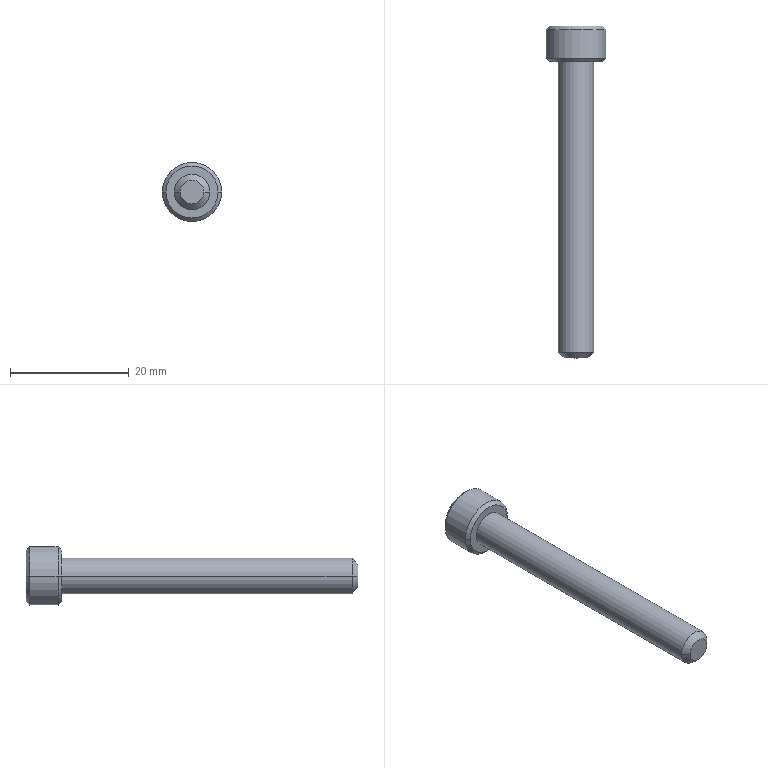Part | STEP file | BB62-M6-50L | 1 solid | 27 faces | box 10 x 56 x 10 mm | volume 1788 mm3 | plane 15 | cone 8 | cylinder 4 | commonest cylinder face diameters 6 x2 10 x2